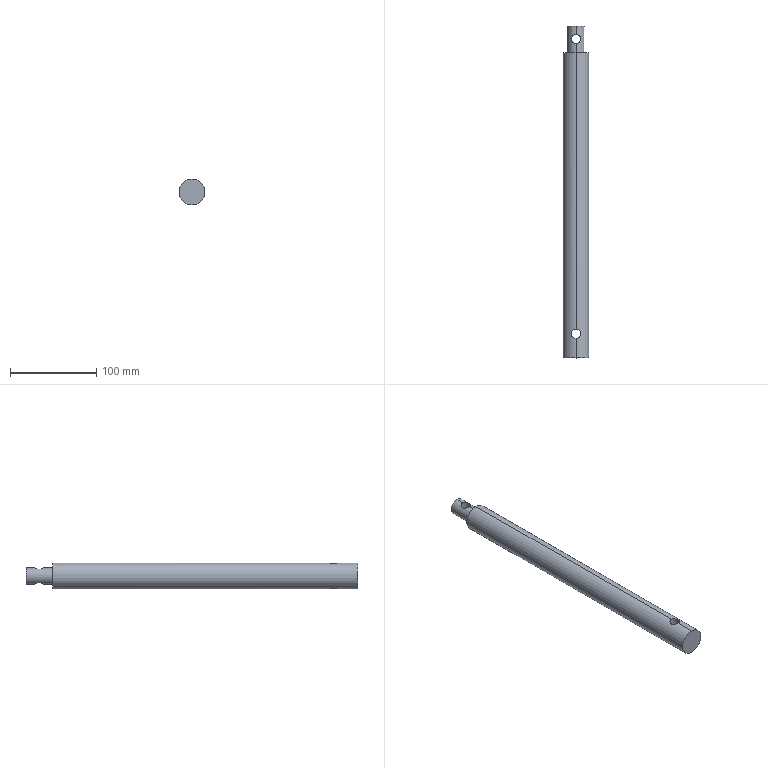Part | SolidWorks | features ICE 2, MoveFace 2, Extrusion 1 | 1 solid | 11 faces | box 30 x 384 x 30 mm | volume 253782 mm3 | cylinder 8 | plane 3 | commonest cylinder face diameters 11 x4 19 x2 30 x2
STEP:
#1=CARTESIAN_POINT('',(-5.5,330.,-13.955));
#2=VERTEX_POINT('',#1);
#3=CARTESIAN_POINT('',(0.,324.5,-15.));
#4=VERTEX_POINT('',#3);
#5=CARTESIAN_POINT('',(-5.5,330.,-13.955));
#6=CARTESIAN_POINT('',(-5.5,329.818,-13.955));
#7=CARTESIAN_POINT('',(-5.491,329.634,-13.959));
#8=CARTESIAN_POINT('',(-5.455,329.272,-13.973));
#9=CARTESIAN_POINT('',(-5.428,329.093,-13.984));
#10=CARTESIAN_POINT('',(-5.321,328.562,-14.025));
#11=CARTESIAN_POINT('',(-5.215,328.214,-14.065));
#12=CARTESIAN_POINT('',(-4.936,327.547,-14.165));
#13=CARTESIAN_POINT('',(-4.766,327.232,-14.224));
#14=CARTESIAN_POINT('',(-4.368,326.639,-14.352));
#15=CARTESIAN_POINT('',(-4.137,326.358,-14.421));
#16=CARTESIAN_POINT('',(-3.633,325.855,-14.556));
#17=CARTESIAN_POINT('',(-3.358,325.63,-14.622));
#18=CARTESIAN_POINT('',(-2.91,325.33,-14.716));
#19=CARTESIAN_POINT('',(-2.755,325.236,-14.746));
#20=CARTESIAN_POINT('',(-2.438,325.067,-14.801));
#21=CARTESIAN_POINT('',(-2.277,324.99,-14.827));
#22=CARTESIAN_POINT('',(-1.782,324.785,-14.897));
#23=CARTESIAN_POINT('',(-1.44,324.679,-14.935));
#24=CARTESIAN_POINT('',(-0.904,324.572,-14.974));
#25=CARTESIAN_POINT('',(-0.7225,324.545,-14.984));
#26=CARTESIAN_POINT('',(-0.3614,324.509,-14.997));
#27=CARTESIAN_POINT('',(-0.1808,324.5,-15.));
#28=CARTESIAN_POINT('',(0.,324.5,-15.));
#29=B_SPLINE_CURVE_WITH_KNOTS('',3,(#5,#6,#7,#8,#9,#10,#11,#12,#13,#14,#15,#16,#17,#18,#19,#20,#21,#22,#23,#24,#25,#26,#27,#28),.UNSPECIFIED.,.F.,.F.,(4,2,2,2,2,2,2,2,2,2,2,4),(0.02696,0.02751,0.02805,0.02913,0.03022,0.0313,0.03239,0.03293,0.03347,0.03456,0.0351,0.03564),.UNSPECIFIED.);
#30=EDGE_CURVE('',#2,#4,#29,.T.);
#31=ORIENTED_EDGE('',*,*,#30,.F.);
#32=CARTESIAN_POINT('',(-5.5,330.,13.955));
#33=VERTEX_POINT('',#32);
#34=CARTESIAN_POINT('',(-5.5,330.,-240.));
#35=DIRECTION('',(0.,0.,1.));
#36=VECTOR('',#35,1000.);
#37=LINE('',#34,#36);
#38=EDGE_CURVE('',#2,#33,#37,.T.);
#39=ORIENTED_EDGE('',*,*,#38,.T.);
#40=CARTESIAN_POINT('',(0.,324.5,15.));
#41=VERTEX_POINT('',#40);
#42=CARTESIAN_POINT('',(0.,324.5,15.));
#43=CARTESIAN_POINT('',(-0.182,324.5,15.));
#44=CARTESIAN_POINT('',(-0.3661,324.509,14.997));
#45=CARTESIAN_POINT('',(-0.7283,324.545,14.983));
#46=CARTESIAN_POINT('',(-0.9072,324.572,14.974));
#47=CARTESIAN_POINT('',(-1.438,324.679,14.935));
#48=CARTESIAN_POINT('',(-1.786,324.785,14.897));
#49=CARTESIAN_POINT('',(-2.454,325.065,14.802));
#50=CARTESIAN_POINT('',(-2.769,325.235,14.745));
#51=CARTESIAN_POINT('',(-3.363,325.633,14.621));
#52=CARTESIAN_POINT('',(-3.643,325.864,14.553));
#53=CARTESIAN_POINT('',(-4.146,326.369,14.418));
#54=CARTESIAN_POINT('',(-4.372,326.643,14.35));
#55=CARTESIAN_POINT('',(-4.671,327.091,14.254));
#56=CARTESIAN_POINT('',(-4.765,327.247,14.223));
#57=CARTESIAN_POINT('',(-4.934,327.563,14.166));
#58=CARTESIAN_POINT('',(-5.01,327.724,14.139));
#59=CARTESIAN_POINT('',(-5.216,328.218,14.065));
#60=CARTESIAN_POINT('',(-5.321,328.561,14.025));
#61=CARTESIAN_POINT('',(-5.428,329.096,13.983));
#62=CARTESIAN_POINT('',(-5.455,329.277,13.973));
#63=CARTESIAN_POINT('',(-5.491,329.639,13.959));
#64=CARTESIAN_POINT('',(-5.5,329.819,13.955));
#65=CARTESIAN_POINT('',(-5.5,330.,13.955));
#66=B_SPLINE_CURVE_WITH_KNOTS('',3,(#42,#43,#44,#45,#46,#47,#48,#49,#50,#51,#52,#53,#54,#55,#56,#57,#58,#59,#60,#61,#62,#63,#64,#65),.UNSPECIFIED.,.F.,.F.,(4,2,2,2,2,2,2,2,2,2,2,4),(0.02696,0.0275,0.02804,0.02912,0.03021,0.03129,0.03238,0.03292,0.03346,0.03455,0.03509,0.03563),.UNSPECIFIED.);
#67=EDGE_CURVE('',#41,#33,#66,.T.);
#68=ORIENTED_EDGE('',*,*,#67,.F.);
#69=CARTESIAN_POINT('',(5.5,330.,13.955));
#70=VERTEX_POINT('',#69);
#71=CARTESIAN_POINT('',(5.5,330.,13.955));
#72=CARTESIAN_POINT('',(5.5,329.634,13.955));
#73=CARTESIAN_POINT('',(5.464,329.275,13.97));
#74=CARTESIAN_POINT('',(5.322,328.566,14.024));
#75=CARTESIAN_POINT('',(5.214,328.214,14.065));
#76=CARTESIAN_POINT('',(4.938,327.551,14.165));
#77=CARTESIAN_POINT('',(4.769,327.236,14.223));
#78=CARTESIAN_POINT('',(4.368,326.638,14.352));
#79=CARTESIAN_POINT('',(4.14,326.361,14.42));
#80=CARTESIAN_POINT('',(3.763,325.984,14.521));
#81=CARTESIAN_POINT('',(3.631,325.865,14.555));
#82=CARTESIAN_POINT('',(3.354,325.638,14.621));
#83=CARTESIAN_POINT('',(3.209,325.529,14.654));
#84=CARTESIAN_POINT('',(2.761,325.23,14.747));
#85=CARTESIAN_POINT('',(2.447,325.061,14.803));
#86=CARTESIAN_POINT('',(1.784,324.785,14.897));
#87=CARTESIAN_POINT('',(1.432,324.677,14.936));
#88=CARTESIAN_POINT('',(0.7232,324.536,14.987));
#89=CARTESIAN_POINT('',(0.364,324.5,15.));
#90=CARTESIAN_POINT('',(0.,324.5,15.));
#91=B_SPLINE_CURVE_WITH_KNOTS('',3,(#71,#72,#73,#74,#75,#76,#77,#78,#79,#80,#81,#82,#83,#84,#85,#86,#87,#88,#89,#90),.UNSPECIFIED.,.F.,.F.,(4,2,2,2,2,2,2,2,2,4),(0.01828,0.01936,0.02045,0.02153,0.02262,0.02316,0.0237,0.02479,0.02587,0.02696),.UNSPECIFIED.);
#92=EDGE_CURVE('',#70,#41,#91,.T.);
#93=ORIENTED_EDGE('',*,*,#92,.F.);
#94=CARTESIAN_POINT('',(5.5,330.,-13.955));
#95=VERTEX_POINT('',#94);
#96=CARTESIAN_POINT('',(5.5,330.,-240.));
#97=DIRECTION('',(0.,0.,1.));
#98=VECTOR('',#97,1000.);
#99=LINE('',#96,#98);
#100=EDGE_CURVE('',#95,#70,#99,.T.);
#101=ORIENTED_EDGE('',*,*,#100,.F.);
#102=CARTESIAN_POINT('',(0.,324.5,-15.));
#103=CARTESIAN_POINT('',(0.1807,324.5,-15.));
#104=CARTESIAN_POINT('',(0.3616,324.509,-14.997));
#105=CARTESIAN_POINT('',(0.7235,324.545,-14.984));
#106=CARTESIAN_POINT('',(0.9054,324.572,-14.974));
#107=CARTESIAN_POINT('',(1.439,324.679,-14.935));
#108=CARTESIAN_POINT('',(1.783,324.785,-14.897));
#109=CARTESIAN_POINT('',(2.448,325.062,-14.803));
#110=CARTESIAN_POINT('',(2.769,325.235,-14.745));
#111=CARTESIAN_POINT('',(3.361,325.632,-14.622));
#112=CARTESIAN_POINT('',(3.637,325.858,-14.555));
#113=CARTESIAN_POINT('',(4.145,326.368,-14.418));
#114=CARTESIAN_POINT('',(4.371,326.643,-14.35));
#115=CARTESIAN_POINT('',(4.668,327.086,-14.255));
#116=CARTESIAN_POINT('',(4.76,327.239,-14.225));
#117=CARTESIAN_POINT('',(4.93,327.556,-14.167));
#118=CARTESIAN_POINT('',(5.009,327.72,-14.139));
#119=CARTESIAN_POINT('',(5.216,328.219,-14.065));
#120=CARTESIAN_POINT('',(5.321,328.562,-14.025));
#121=CARTESIAN_POINT('',(5.463,329.27,-13.97));
#122=CARTESIAN_POINT('',(5.5,329.638,-13.955));
#123=CARTESIAN_POINT('',(5.5,330.,-13.955));
#124=B_SPLINE_CURVE_WITH_KNOTS('',3,(#102,#103,#104,#105,#106,#107,#108,#109,#110,#111,#112,#113,#114,#115,#116,#117,#118,#119,#120,#121,#122,#123),.UNSPECIFIED.,.F.,.F.,(4,2,2,2,2,2,2,2,2,2,4),(0.0009354,0.001478,0.00202,0.003104,0.004189,0.005273,0.006357,0.006899,0.007442,0.008526,0.00961),.UNSPECIFIED.);
#125=EDGE_CURVE('',#4,#95,#124,.T.);
#126=ORIENTED_EDGE('',*,*,#125,.F.);
#127=EDGE_LOOP('',(#31,#39,#68,#93,#101,#126));
#128=FACE_OUTER_BOUND('',#127,.T.);
#129=CARTESIAN_POINT('',(0.,330.,-240.));
#130=DIRECTION('',(0.,0.,1.));
#131=DIRECTION('',(1.,0.,0.));
#132=AXIS2_PLACEMENT_3D('',#129,#130,#131);
#133=CYLINDRICAL_SURFACE('',#132,5.5);
#134=ADVANCED_FACE('',(#128),#133,.F.);
#135=CARTESIAN_POINT('',(-5.5,671.,-7.746));
#136=VERTEX_POINT('',#135);
#137=CARTESIAN_POINT('',(0.,665.5,-9.5));
#138=VERTEX_POINT('',#137);
#139=CARTESIAN_POINT('',(-5.5,671.,-7.746));
#140=CARTESIAN_POINT('',(-5.5,670.628,-7.746));
#141=CARTESIAN_POINT('',(-5.463,670.263,-7.773));
#142=CARTESIAN_POINT('',(-5.317,669.547,-7.873));
#143=CARTESIAN_POINT('',(-5.208,669.195,-7.947));
#144=CARTESIAN_POINT('',(-4.93,668.535,-8.122));
#145=CARTESIAN_POINT('',(-4.759,668.22,-8.225));
#146=CARTESIAN_POINT('',(-4.363,667.633,-8.442));
#147=CARTESIAN_POINT('',(-4.141,667.363,-8.555));
#148=CARTESIAN_POINT('',(-3.644,666.865,-8.778));
#149=CARTESIAN_POINT('',(-3.368,666.637,-8.888));
#150=CARTESIAN_POINT('',(-2.782,666.242,-9.089));
#151=CARTESIAN_POINT('',(-2.47,666.073,-9.18));
#152=CARTESIAN_POINT('',(-1.971,665.862,-9.295));
#153=CARTESIAN_POINT('',(-1.798,665.799,-9.33));
#154=CARTESIAN_POINT('',(-1.449,665.691,-9.39));
#155=CARTESIAN_POINT('',(-1.273,665.646,-9.416));
#156=CARTESIAN_POINT('',(-0.7385,665.538,-9.478));
#157=CARTESIAN_POINT('',(-0.3726,665.5,-9.5));
#158=CARTESIAN_POINT('',(0.,665.5,-9.5));
#159=B_SPLINE_CURVE_WITH_KNOTS('',3,(#139,#140,#141,#142,#143,#144,#145,#146,#147,#148,#149,#150,#151,#152,#153,#154,#155,#156,#157,#158),.UNSPECIFIED.,.F.,.F.,(4,2,2,2,2,2,2,2,2,4),(0.008806,0.009907,0.01101,0.01211,0.01321,0.01431,0.01541,0.01596,0.01651,0.01761),.UNSPECIFIED.);
#160=EDGE_CURVE('',#136,#138,#159,.T.);
#161=ORIENTED_EDGE('',*,*,#160,.F.);
#162=CARTESIAN_POINT('',(-5.5,671.,7.746));
#163=VERTEX_POINT('',#162);
#164=CARTESIAN_POINT('',(-5.5,671.,-240.));
#165=DIRECTION('',(0.,0.,1.));
#166=VECTOR('',#165,1000.);
#167=LINE('',#164,#166);
#168=EDGE_CURVE('',#136,#163,#167,.T.);
#169=ORIENTED_EDGE('',*,*,#168,.T.);
#170=CARTESIAN_POINT('',(0.,665.5,9.5));
#171=VERTEX_POINT('',#170);
#172=CARTESIAN_POINT('',(0.,665.5,9.5));
#173=CARTESIAN_POINT('',(-0.1848,665.5,9.5));
#174=CARTESIAN_POINT('',(-0.3717,665.509,9.495));
#175=CARTESIAN_POINT('',(-0.7383,665.547,9.473));
#176=CARTESIAN_POINT('',(-0.9194,665.574,9.457));
#177=CARTESIAN_POINT('',(-1.277,665.647,9.416));
#178=CARTESIAN_POINT('',(-1.454,665.692,9.39));
#179=CARTESIAN_POINT('',(-1.802,665.801,9.329));
#180=CARTESIAN_POINT('',(-1.975,665.864,9.294));
#181=CARTESIAN_POINT('',(-2.474,666.074,9.179));
#182=CARTESIAN_POINT('',(-2.787,666.245,9.087));
#183=CARTESIAN_POINT('',(-3.377,666.644,8.885));
#184=CARTESIAN_POINT('',(-3.65,666.871,8.775));
#185=CARTESIAN_POINT('',(-4.145,667.368,8.552));
#186=CARTESIAN_POINT('',(-4.37,667.641,8.438));
#187=CARTESIAN_POINT('',(-4.764,668.229,8.222));
#188=CARTESIAN_POINT('',(-4.932,668.539,8.121));
#189=CARTESIAN_POINT('',(-5.139,669.031,7.991));
#190=CARTESIAN_POINT('',(-5.2,669.2,7.951));
#191=CARTESIAN_POINT('',(-5.308,669.547,7.879));
#192=CARTESIAN_POINT('',(-5.353,669.725,7.848));
#193=CARTESIAN_POINT('',(-5.463,670.263,7.773));
#194=CARTESIAN_POINT('',(-5.5,670.628,7.746));
#195=CARTESIAN_POINT('',(-5.5,671.,7.746));
#196=B_SPLINE_CURVE_WITH_KNOTS('',3,(#172,#173,#174,#175,#176,#177,#178,#179,#180,#181,#182,#183,#184,#185,#186,#187,#188,#189,#190,#191,#192,#193,#194,#195),.UNSPECIFIED.,.F.,.F.,(4,2,2,2,2,2,2,2,2,2,2,4),(0.00881,0.00936,0.009909,0.01046,0.01101,0.01211,0.01321,0.01431,0.01541,0.01595,0.0165,0.0176),.UNSPECIFIED.);
#197=EDGE_CURVE('',#171,#163,#196,.T.);
#198=ORIENTED_EDGE('',*,*,#197,.F.);
#199=CARTESIAN_POINT('',(5.5,671.,7.746));
#200=VERTEX_POINT('',#199);
#201=CARTESIAN_POINT('',(5.5,671.,7.746));
#202=CARTESIAN_POINT('',(5.5,670.627,7.746));
#203=CARTESIAN_POINT('',(5.462,670.262,7.773));
#204=CARTESIAN_POINT('',(5.317,669.548,7.873));
#205=CARTESIAN_POINT('',(5.208,669.196,7.947));
#206=CARTESIAN_POINT('',(4.93,668.535,8.122));
#207=CARTESIAN_POINT('',(4.761,668.224,8.224));
#208=CARTESIAN_POINT('',(4.363,667.633,8.442));
#209=CARTESIAN_POINT('',(4.14,667.362,8.555));
#210=CARTESIAN_POINT('',(3.768,666.99,8.722));
#211=CARTESIAN_POINT('',(3.638,666.871,8.777));
#212=CARTESIAN_POINT('',(3.365,666.646,8.885));
#213=CARTESIAN_POINT('',(3.221,666.538,8.939));
#214=CARTESIAN_POINT('',(2.78,666.241,9.09));
#215=CARTESIAN_POINT('',(2.468,666.072,9.18));
#216=CARTESIAN_POINT('',(1.805,665.792,9.333));
#217=CARTESIAN_POINT('',(1.451,665.682,9.396));
#218=CARTESIAN_POINT('',(0.7344,665.537,9.478));
#219=CARTESIAN_POINT('',(0.3703,665.5,9.5));
#220=CARTESIAN_POINT('',(0.,665.5,9.5));
#221=B_SPLINE_CURVE_WITH_KNOTS('',3,(#201,#202,#203,#204,#205,#206,#207,#208,#209,#210,#211,#212,#213,#214,#215,#216,#217,#218,#219,#220),.UNSPECIFIED.,.F.,.F.,(4,2,2,2,2,2,2,2,2,4),(0.,0.001101,0.002203,0.003304,0.004405,0.004956,0.005506,0.006608,0.007709,0.00881),.UNSPECIFIED.);
#222=EDGE_CURVE('',#200,#171,#221,.T.);
#223=ORIENTED_EDGE('',*,*,#222,.F.);
#224=CARTESIAN_POINT('',(5.5,671.,-7.746));
#225=VERTEX_POINT('',#224);
#226=CARTESIAN_POINT('',(5.5,671.,-240.));
#227=DIRECTION('',(0.,0.,1.));
#228=VECTOR('',#227,1000.);
#229=LINE('',#226,#228);
#230=EDGE_CURVE('',#225,#200,#229,.T.);
#231=ORIENTED_EDGE('',*,*,#230,.F.);
#232=CARTESIAN_POINT('',(0.,665.5,-9.5));
#233=CARTESIAN_POINT('',(0.372,665.5,-9.5));
#234=CARTESIAN_POINT('',(0.7369,665.537,-9.478));
#235=CARTESIAN_POINT('',(1.453,665.683,-9.395));
#236=CARTESIAN_POINT('',(1.807,665.793,-9.333));
#237=CARTESIAN_POINT('',(2.471,666.073,-9.179));
#238=CARTESIAN_POINT('',(2.785,666.244,-9.088));
#239=CARTESIAN_POINT('',(3.377,666.644,-8.885));
#240=CARTESIAN_POINT('',(3.648,666.869,-8.776));
#241=CARTESIAN_POINT('',(4.143,667.366,-8.553));
#242=CARTESIAN_POINT('',(4.369,667.641,-8.439));
#243=CARTESIAN_POINT('',(4.762,668.225,-8.224));
#244=CARTESIAN_POINT('',(4.929,668.535,-8.123));
#245=CARTESIAN_POINT('',(5.207,669.194,-7.947));
#246=CARTESIAN_POINT('',(5.317,669.545,-7.873));
#247=CARTESIAN_POINT('',(5.426,670.081,-7.798));
#248=CARTESIAN_POINT('',(5.453,670.262,-7.779));
#249=CARTESIAN_POINT('',(5.49,670.628,-7.753));
#250=CARTESIAN_POINT('',(5.5,670.815,-7.746));
#251=CARTESIAN_POINT('',(5.5,671.,-7.746));
#252=B_SPLINE_CURVE_WITH_KNOTS('',3,(#232,#233,#234,#235,#236,#237,#238,#239,#240,#241,#242,#243,#244,#245,#246,#247,#248,#249,#250,#251),.UNSPECIFIED.,.F.,.F.,(4,2,2,2,2,2,2,2,2,4),(0.01761,0.01871,0.01981,0.02091,0.022,0.0231,0.0242,0.0253,0.02585,0.0264),.UNSPECIFIED.);
#253=EDGE_CURVE('',#138,#225,#252,.T.);
#254=ORIENTED_EDGE('',*,*,#253,.F.);
#255=EDGE_LOOP('',(#161,#169,#198,#223,#231,#254));
#256=FACE_OUTER_BOUND('',#255,.T.);
#257=CARTESIAN_POINT('',(0.,671.,-240.));
#258=DIRECTION('',(0.,0.,1.));
#259=DIRECTION('',(1.,0.,0.));
#260=AXIS2_PLACEMENT_3D('',#257,#258,#259);
#261=CYLINDRICAL_SURFACE('',#260,5.5);
#262=ADVANCED_FACE('',(#256),#261,.F.);
#263=CARTESIAN_POINT('',(0.,686.,9.5));
#264=VERTEX_POINT('',#263);
#265=CARTESIAN_POINT('',(0.,686.,-9.5));
#266=VERTEX_POINT('',#265);
#267=CARTESIAN_POINT('',(0.,686.,0.));
#268=DIRECTION('',(0.,1.,0.));
#269=DIRECTION('',(0.,0.,1.));
#270=AXIS2_PLACEMENT_3D('',#267,#268,#269);
#271=CIRCLE('',#270,9.5);
#272=EDGE_CURVE('',#264,#266,#271,.T.);
#273=ORIENTED_EDGE('',*,*,#272,.F.);
#274=CARTESIAN_POINT('',(0.,676.5,9.5));
#275=VERTEX_POINT('',#274);
#276=CARTESIAN_POINT('',(0.,686.,9.5));
#277=DIRECTION('',(0.,-1.,0.));
#278=VECTOR('',#277,1000.);
#279=LINE('',#276,#278);
#280=EDGE_CURVE('',#264,#275,#279,.T.);
#281=ORIENTED_EDGE('',*,*,#280,.T.);
#282=CARTESIAN_POINT('',(0.,676.5,9.5));
#283=CARTESIAN_POINT('',(0.3713,676.5,9.5));
#284=CARTESIAN_POINT('',(0.7393,676.462,9.478));
#285=CARTESIAN_POINT('',(1.455,676.317,9.395));
#286=CARTESIAN_POINT('',(1.808,676.207,9.333));
#287=CARTESIAN_POINT('',(2.473,675.926,9.179));
#288=CARTESIAN_POINT('',(2.786,675.756,9.088));
#289=CARTESIAN_POINT('',(3.378,675.355,8.885));
#290=CARTESIAN_POINT('',(3.65,675.129,8.775));
#291=CARTESIAN_POINT('',(4.021,674.757,8.608));
#292=CARTESIAN_POINT('',(4.139,674.627,8.552));
#293=CARTESIAN_POINT('',(4.362,674.354,8.44));
#294=CARTESIAN_POINT('',(4.469,674.211,8.384));
#295=CARTESIAN_POINT('',(4.763,673.772,8.223));
#296=CARTESIAN_POINT('',(4.931,673.462,8.122));
#297=CARTESIAN_POINT('',(5.208,672.805,7.947));
#298=CARTESIAN_POINT('',(5.317,672.453,7.873));
#299=CARTESIAN_POINT('',(5.462,671.738,7.773));
#300=CARTESIAN_POINT('',(5.5,671.372,7.746));
#301=CARTESIAN_POINT('',(5.5,671.,7.746));
#302=B_SPLINE_CURVE_WITH_KNOTS('',3,(#282,#283,#284,#285,#286,#287,#288,#289,#290,#291,#292,#293,#294,#295,#296,#297,#298,#299,#300,#301),.UNSPECIFIED.,.F.,.F.,(4,2,2,2,2,2,2,2,2,4),(0.02639,0.02749,0.02859,0.02969,0.03078,0.03133,0.03188,0.03298,0.03408,0.03517),.UNSPECIFIED.);
#303=EDGE_CURVE('',#275,#200,#302,.T.);
#304=ORIENTED_EDGE('',*,*,#303,.T.);
#305=ORIENTED_EDGE('',*,*,#222,.T.);
#306=CARTESIAN_POINT('',(0.,655.,9.5));
#307=VERTEX_POINT('',#306);
#308=CARTESIAN_POINT('',(0.,686.,9.5));
#309=DIRECTION('',(0.,-1.,0.));
#310=VECTOR('',#309,1000.);
#311=LINE('',#308,#310);
#312=EDGE_CURVE('',#171,#307,#311,.T.);
#313=ORIENTED_EDGE('',*,*,#312,.T.);
#314=CARTESIAN_POINT('',(0.,655.,-9.5));
#315=VERTEX_POINT('',#314);
#316=CARTESIAN_POINT('',(0.,655.,0.));
#317=DIRECTION('',(0.,1.,0.));
#318=DIRECTION('',(0.,0.,1.));
#319=AXIS2_PLACEMENT_3D('',#316,#317,#318);
#320=CIRCLE('',#319,9.5);
#321=EDGE_CURVE('',#307,#315,#320,.T.);
#322=ORIENTED_EDGE('',*,*,#321,.T.);
#323=CARTESIAN_POINT('',(0.,686.,-9.5));
#324=DIRECTION('',(0.,-1.,0.));
#325=VECTOR('',#324,1000.);
#326=LINE('',#323,#325);
#327=EDGE_CURVE('',#138,#315,#326,.T.);
#328=ORIENTED_EDGE('',*,*,#327,.F.);
#329=ORIENTED_EDGE('',*,*,#253,.T.);
#330=CARTESIAN_POINT('',(0.,676.5,-9.5));
#331=VERTEX_POINT('',#330);
#332=CARTESIAN_POINT('',(5.5,671.,-7.746));
#333=CARTESIAN_POINT('',(5.5,671.37,-7.746));
#334=CARTESIAN_POINT('',(5.463,671.734,-7.773));
#335=CARTESIAN_POINT('',(5.354,672.272,-7.848));
#336=CARTESIAN_POINT('',(5.308,672.451,-7.879));
#337=CARTESIAN_POINT('',(5.201,672.797,-7.95));
#338=CARTESIAN_POINT('',(5.14,672.966,-7.99));
#339=CARTESIAN_POINT('',(4.932,673.461,-8.121));
#340=CARTESIAN_POINT('',(4.76,673.777,-8.224));
#341=CARTESIAN_POINT('',(4.367,674.363,-8.44));
#342=CARTESIAN_POINT('',(4.144,674.633,-8.553));
#343=CARTESIAN_POINT('',(3.771,675.007,-8.72));
#344=CARTESIAN_POINT('',(3.64,675.127,-8.776));
#345=CARTESIAN_POINT('',(3.368,675.352,-8.884));
#346=CARTESIAN_POINT('',(3.227,675.457,-8.937));
#347=CARTESIAN_POINT('',(2.789,675.754,-9.087));
#348=CARTESIAN_POINT('',(2.477,675.924,-9.178));
#349=CARTESIAN_POINT('',(1.809,676.207,-9.333));
#350=CARTESIAN_POINT('',(1.46,676.315,-9.394));
#351=CARTESIAN_POINT('',(0.7444,676.462,-9.478));
#352=CARTESIAN_POINT('',(0.3717,676.5,-9.5));
#353=CARTESIAN_POINT('',(0.,676.5,-9.5));
#354=B_SPLINE_CURVE_WITH_KNOTS('',3,(#332,#333,#334,#335,#336,#337,#338,#339,#340,#341,#342,#343,#344,#345,#346,#347,#348,#349,#350,#351,#352,#353),.UNSPECIFIED.,.F.,.F.,(4,2,2,2,2,2,2,2,2,2,4),(0.0264,0.0275,0.02804,0.02859,0.02969,0.03079,0.03134,0.03189,0.03298,0.03408,0.03518),.UNSPECIFIED.);
#355=EDGE_CURVE('',#225,#331,#354,.T.);
#356=ORIENTED_EDGE('',*,*,#355,.T.);
#357=CARTESIAN_POINT('',(0.,686.,-9.5));
#358=DIRECTION('',(0.,-1.,0.));
#359=VECTOR('',#358,1000.);
#360=LINE('',#357,#359);
#361=EDGE_CURVE('',#266,#331,#360,.T.);
#362=ORIENTED_EDGE('',*,*,#361,.F.);
#363=EDGE_LOOP('',(#273,#281,#304,#305,#313,#322,#328,#329,#356,#362));
#364=FACE_OUTER_BOUND('',#363,.T.);
#365=CARTESIAN_POINT('',(0.,686.,0.));
#366=DIRECTION('',(0.,-1.,0.));
#367=DIRECTION('',(0.,0.,-1.));
#368=AXIS2_PLACEMENT_3D('',#365,#366,#367);
#369=CYLINDRICAL_SURFACE('',#368,9.5);
#370=ADVANCED_FACE('',(#364),#369,.T.);
#371=CARTESIAN_POINT('',(0.,655.,15.));
#372=VERTEX_POINT('',#371);
#373=CARTESIAN_POINT('',(0.,655.,-15.));
#374=VERTEX_POINT('',#373);
#375=CARTESIAN_POINT('',(0.,655.,0.));
#376=DIRECTION('',(0.,1.,0.));
#377=DIRECTION('',(0.,0.,1.));
#378=AXIS2_PLACEMENT_3D('',#375,#376,#377);
#379=CIRCLE('',#378,15.);
#380=EDGE_CURVE('',#372,#374,#379,.T.);
#381=ORIENTED_EDGE('',*,*,#380,.F.);
#382=CARTESIAN_POINT('',(0.,335.5,15.));
#383=VERTEX_POINT('',#382);
#384=CARTESIAN_POINT('',(0.,656.,15.));
#385=DIRECTION('',(0.,-1.,0.));
#386=VECTOR('',#385,1000.);
#387=LINE('',#384,#386);
#388=EDGE_CURVE('',#372,#383,#387,.T.);
#389=ORIENTED_EDGE('',*,*,#388,.T.);
#390=CARTESIAN_POINT('',(0.,335.5,15.));
#391=CARTESIAN_POINT('',(0.3621,335.5,15.));
#392=CARTESIAN_POINT('',(0.7219,335.465,14.987));
#393=CARTESIAN_POINT('',(1.258,335.357,14.948));
#394=CARTESIAN_POINT('',(1.435,335.313,14.932));
#395=CARTESIAN_POINT('',(1.781,335.207,14.895));
#396=CARTESIAN_POINT('',(1.95,335.146,14.874));
#397=CARTESIAN_POINT('',(2.281,335.008,14.826));
#398=CARTESIAN_POINT('',(2.443,334.931,14.801));
#399=CARTESIAN_POINT('',(2.76,334.76,14.745));
#400=CARTESIAN_POINT('',(2.916,334.667,14.715));
#401=CARTESIAN_POINT('',(3.363,334.367,14.621));
#402=CARTESIAN_POINT('',(3.637,334.141,14.555));
#403=CARTESIAN_POINT('',(4.142,333.636,14.419));
#404=CARTESIAN_POINT('',(4.372,333.356,14.35));
#405=CARTESIAN_POINT('',(4.768,332.764,14.223));
#406=CARTESIAN_POINT('',(4.937,332.45,14.165));
#407=CARTESIAN_POINT('',(5.146,331.949,14.09));
#408=CARTESIAN_POINT('',(5.208,331.778,14.067));
#409=CARTESIAN_POINT('',(5.313,331.433,14.028));
#410=CARTESIAN_POINT('',(5.401,331.084,13.994));
#411=CARTESIAN_POINT('',(5.455,330.727,13.973));
#412=CARTESIAN_POINT('',(5.491,330.366,13.959));
#413=CARTESIAN_POINT('',(5.5,330.183,13.955));
#414=CARTESIAN_POINT('',(5.5,330.,13.955));
#415=B_SPLINE_CURVE_WITH_KNOTS('',3,(#390,#391,#392,#393,#394,#395,#396,#397,#398,#399,#400,#401,#402,#403,#404,#405,#406,#407,#408,#409,#410,#411,#412,#413,#414),.UNSPECIFIED.,.F.,.F.,(4,2,2,2,2,2,2,2,2,2,1,2,4),(0.009602,0.01069,0.01123,0.01177,0.01231,0.01286,0.01394,0.01503,0.01611,0.01665,0.01719,0.01774,0.01828),.UNSPECIFIED.);
#416=EDGE_CURVE('',#383,#70,#415,.T.);
#417=ORIENTED_EDGE('',*,*,#416,.T.);
#418=ORIENTED_EDGE('',*,*,#92,.T.);
#419=CARTESIAN_POINT('',(0.,302.,15.));
#420=VERTEX_POINT('',#419);
#421=CARTESIAN_POINT('',(0.,656.,15.));
#422=DIRECTION('',(0.,-1.,0.));
#423=VECTOR('',#422,1000.);
#424=LINE('',#421,#423);
#425=EDGE_CURVE('',#41,#420,#424,.T.);
#426=ORIENTED_EDGE('',*,*,#425,.T.);
#427=CARTESIAN_POINT('',(0.,302.,-15.));
#428=VERTEX_POINT('',#427);
#429=CARTESIAN_POINT('',(0.,302.,0.));
#430=DIRECTION('',(0.,1.,0.));
#431=DIRECTION('',(0.,0.,1.));
#432=AXIS2_PLACEMENT_3D('',#429,#430,#431);
#433=CIRCLE('',#432,15.);
#434=EDGE_CURVE('',#420,#428,#433,.T.);
#435=ORIENTED_EDGE('',*,*,#434,.T.);
#436=CARTESIAN_POINT('',(0.,656.,-15.));
#437=DIRECTION('',(0.,-1.,0.));
#438=VECTOR('',#437,1000.);
#439=LINE('',#436,#438);
#440=EDGE_CURVE('',#4,#428,#439,.T.);
#441=ORIENTED_EDGE('',*,*,#440,.F.);
#442=ORIENTED_EDGE('',*,*,#125,.T.);
#443=CARTESIAN_POINT('',(0.,335.5,-15.));
#444=VERTEX_POINT('',#443);
#445=CARTESIAN_POINT('',(5.5,330.,-13.955));
#446=CARTESIAN_POINT('',(5.5,330.362,-13.955));
#447=CARTESIAN_POINT('',(5.465,330.722,-13.969));
#448=CARTESIAN_POINT('',(5.357,331.257,-14.011));
#449=CARTESIAN_POINT('',(5.313,331.435,-14.028));
#450=CARTESIAN_POINT('',(5.207,331.78,-14.067));
#451=CARTESIAN_POINT('',(5.146,331.949,-14.09));
#452=CARTESIAN_POINT('',(5.008,332.28,-14.139));
#453=CARTESIAN_POINT('',(4.931,332.442,-14.167));
#454=CARTESIAN_POINT('',(4.761,332.759,-14.225));
#455=CARTESIAN_POINT('',(4.668,332.915,-14.256));
#456=CARTESIAN_POINT('',(4.368,333.361,-14.351));
#457=CARTESIAN_POINT('',(4.142,333.636,-14.419));
#458=CARTESIAN_POINT('',(3.638,334.14,-14.554));
#459=CARTESIAN_POINT('',(3.358,334.371,-14.622));
#460=CARTESIAN_POINT('',(2.765,334.768,-14.746));
#461=CARTESIAN_POINT('',(2.451,334.937,-14.802));
#462=CARTESIAN_POINT('',(1.95,335.146,-14.874));
#463=CARTESIAN_POINT('',(1.778,335.208,-14.895));
#464=CARTESIAN_POINT('',(1.433,335.313,-14.932));
#465=CARTESIAN_POINT('',(1.084,335.401,-14.964));
#466=CARTESIAN_POINT('',(0.7269,335.455,-14.983));
#467=CARTESIAN_POINT('',(0.3661,335.491,-14.997));
#468=CARTESIAN_POINT('',(0.1827,335.5,-15.));
#469=CARTESIAN_POINT('',(0.,335.5,-15.));
#470=B_SPLINE_CURVE_WITH_KNOTS('',3,(#445,#446,#447,#448,#449,#450,#451,#452,#453,#454,#455,#456,#457,#458,#459,#460,#461,#462,#463,#464,#465,#466,#467,#468,#469),.UNSPECIFIED.,.F.,.F.,(4,2,2,2,2,2,2,2,2,2,1,2,4),(0.00961,0.01069,0.01124,0.01178,0.01232,0.01286,0.01395,0.01503,0.01612,0.01666,0.0172,0.01774,0.01829),.UNSPECIFIED.);
#471=EDGE_CURVE('',#95,#444,#470,.T.);
#472=ORIENTED_EDGE('',*,*,#471,.T.);
#473=CARTESIAN_POINT('',(0.,656.,-15.));
#474=DIRECTION('',(0.,-1.,0.));
#475=VECTOR('',#474,1000.);
#476=LINE('',#473,#475);
#477=EDGE_CURVE('',#374,#444,#476,.T.);
#478=ORIENTED_EDGE('',*,*,#477,.F.);
#479=EDGE_LOOP('',(#381,#389,#417,#418,#426,#435,#441,#442,#472,#478));
#480=FACE_OUTER_BOUND('',#479,.T.);
#481=CARTESIAN_POINT('',(0.,656.,0.));
#482=DIRECTION('',(0.,-1.,0.));
#483=DIRECTION('',(0.,0.,-1.));
#484=AXIS2_PLACEMENT_3D('',#481,#482,#483);
#485=CYLINDRICAL_SURFACE('',#484,15.);
#486=ADVANCED_FACE('',(#480),#485,.T.);
#487=ORIENTED_EDGE('',*,*,#388,.F.);
#488=CARTESIAN_POINT('',(0.,655.,0.));
#489=DIRECTION('',(0.,1.,0.));
#490=DIRECTION('',(0.,0.,1.));
#491=AXIS2_PLACEMENT_3D('',#488,#489,#490);
#492=CIRCLE('',#491,15.);
#493=EDGE_CURVE('',#374,#372,#492,.T.);
#494=ORIENTED_EDGE('',*,*,#493,.F.);
#495=ORIENTED_EDGE('',*,*,#477,.T.);
#496=CARTESIAN_POINT('',(0.,335.5,-15.));
#497=CARTESIAN_POINT('',(-0.3655,335.5,-15.));
#498=CARTESIAN_POINT('',(-0.7254,335.464,-14.987));
#499=CARTESIAN_POINT('',(-1.434,335.322,-14.935));
#500=CARTESIAN_POINT('',(-1.786,335.214,-14.897));
#501=CARTESIAN_POINT('',(-2.45,334.937,-14.802));
#502=CARTESIAN_POINT('',(-2.765,334.768,-14.746));
#503=CARTESIAN_POINT('',(-3.363,334.367,-14.621));
#504=CARTESIAN_POINT('',(-3.64,334.138,-14.554));
#505=CARTESIAN_POINT('',(-4.017,333.761,-14.453));
#506=CARTESIAN_POINT('',(-4.137,333.629,-14.419));
#507=CARTESIAN_POINT('',(-4.364,333.353,-14.352));
#508=CARTESIAN_POINT('',(-4.472,333.207,-14.318));
#509=CARTESIAN_POINT('',(-4.771,332.76,-14.223));
#510=CARTESIAN_POINT('',(-4.939,332.445,-14.164));
#511=CARTESIAN_POINT('',(-5.215,331.784,-14.065));
#512=CARTESIAN_POINT('',(-5.323,331.432,-14.024));
#513=CARTESIAN_POINT('',(-5.464,330.723,-13.97));
#514=CARTESIAN_POINT('',(-5.5,330.364,-13.955));
#515=CARTESIAN_POINT('',(-5.5,330.,-13.955));
#516=B_SPLINE_CURVE_WITH_KNOTS('',3,(#496,#497,#498,#499,#500,#501,#502,#503,#504,#505,#506,#507,#508,#509,#510,#511,#512,#513,#514,#515),.UNSPECIFIED.,.F.,.F.,(4,2,2,2,2,2,2,2,2,4),(0.01829,0.01937,0.02046,0.02154,0.02263,0.02317,0.02371,0.02479,0.02588,0.02696),.UNSPECIFIED.);
#517=EDGE_CURVE('',#444,#2,#516,.T.);
#518=ORIENTED_EDGE('',*,*,#517,.T.);
#519=ORIENTED_EDGE('',*,*,#30,.T.);
#520=ORIENTED_EDGE('',*,*,#440,.T.);
#521=CARTESIAN_POINT('',(0.,302.,0.));
#522=DIRECTION('',(0.,1.,0.));
#523=DIRECTION('',(0.,0.,1.));
#524=AXIS2_PLACEMENT_3D('',#521,#522,#523);
#525=CIRCLE('',#524,15.);
#526=EDGE_CURVE('',#428,#420,#525,.T.);
#527=ORIENTED_EDGE('',*,*,#526,.T.);
#528=ORIENTED_EDGE('',*,*,#425,.F.);
#529=ORIENTED_EDGE('',*,*,#67,.T.);
#530=CARTESIAN_POINT('',(-5.5,330.,13.955));
#531=CARTESIAN_POINT('',(-5.5,330.181,13.955));
#532=CARTESIAN_POINT('',(-5.491,330.362,13.959));
#533=CARTESIAN_POINT('',(-5.455,330.723,13.973));
#534=CARTESIAN_POINT('',(-5.428,330.905,13.983));
#535=CARTESIAN_POINT('',(-5.321,331.439,14.025));
#536=CARTESIAN_POINT('',(-5.215,331.783,14.065));
#537=CARTESIAN_POINT('',(-4.939,332.447,14.164));
#538=CARTESIAN_POINT('',(-4.766,332.768,14.224));
#539=CARTESIAN_POINT('',(-4.369,333.36,14.351));
#540=CARTESIAN_POINT('',(-4.143,333.635,14.419));
#541=CARTESIAN_POINT('',(-3.634,334.144,14.556));
#542=CARTESIAN_POINT('',(-3.359,334.37,14.622));
#543=CARTESIAN_POINT('',(-2.915,334.667,14.715));
#544=CARTESIAN_POINT('',(-2.762,334.76,14.744));
#545=CARTESIAN_POINT('',(-2.445,334.93,14.8));
#546=CARTESIAN_POINT('',(-2.281,335.008,14.827));
#547=CARTESIAN_POINT('',(-1.781,335.216,14.898));
#548=CARTESIAN_POINT('',(-1.438,335.321,14.935));
#549=CARTESIAN_POINT('',(-0.7301,335.463,14.986));
#550=CARTESIAN_POINT('',(-0.3621,335.5,15.));
#551=CARTESIAN_POINT('',(0.,335.5,15.));
#552=B_SPLINE_CURVE_WITH_KNOTS('',3,(#530,#531,#532,#533,#534,#535,#536,#537,#538,#539,#540,#541,#542,#543,#544,#545,#546,#547,#548,#549,#550,#551),.UNSPECIFIED.,.F.,.F.,(4,2,2,2,2,2,2,2,2,2,4),(0.0009274,0.00147,0.002012,0.003096,0.00418,0.005265,0.006349,0.006891,0.007434,0.008518,0.009602),.UNSPECIFIED.);
#553=EDGE_CURVE('',#33,#383,#552,.T.);
#554=ORIENTED_EDGE('',*,*,#553,.T.);
#555=EDGE_LOOP('',(#487,#494,#495,#518,#519,#520,#527,#528,#529,#554));
#556=FACE_OUTER_BOUND('',#555,.T.);
#557=CARTESIAN_POINT('',(0.,656.,0.));
#558=DIRECTION('',(0.,-1.,0.));
#559=DIRECTION('',(0.,0.,-1.));
#560=AXIS2_PLACEMENT_3D('',#557,#558,#559);
#561=CYLINDRICAL_SURFACE('',#560,15.);
#562=ADVANCED_FACE('',(#556),#561,.T.);
#563=CARTESIAN_POINT('',(0.,655.,0.));
#564=DIRECTION('',(0.,1.,0.));
#565=DIRECTION('',(0.,0.,1.));
#566=AXIS2_PLACEMENT_3D('',#563,#564,#565);
#567=CIRCLE('',#566,9.5);
#568=EDGE_CURVE('',#315,#307,#567,.T.);
#569=ORIENTED_EDGE('',*,*,#568,.F.);
#570=ORIENTED_EDGE('',*,*,#321,.F.);
#571=EDGE_LOOP('',(#569,#570));
#572=FACE_BOUND('',#571,.T.);
#573=ORIENTED_EDGE('',*,*,#493,.T.);
#574=ORIENTED_EDGE('',*,*,#380,.T.);
#575=EDGE_LOOP('',(#573,#574));
#576=FACE_OUTER_BOUND('',#575,.T.);
#577=CARTESIAN_POINT('',(0.,655.,0.));
#578=DIRECTION('',(0.,1.,0.));
#579=DIRECTION('',(0.,0.,1.));
#580=AXIS2_PLACEMENT_3D('',#577,#578,#579);
#581=PLANE('',#580);
#582=ADVANCED_FACE('',(#572,#576),#581,.T.);
#583=ORIENTED_EDGE('',*,*,#526,.F.);
#584=ORIENTED_EDGE('',*,*,#434,.F.);
#585=EDGE_LOOP('',(#583,#584));
#586=FACE_OUTER_BOUND('',#585,.T.);
#587=CARTESIAN_POINT('',(0.,302.,0.));
#588=DIRECTION('',(0.,1.,0.));
#589=DIRECTION('',(0.,0.,1.));
#590=AXIS2_PLACEMENT_3D('',#587,#588,#589);
#591=PLANE('',#590);
#592=ADVANCED_FACE('',(#586),#591,.F.);
#593=ORIENTED_EDGE('',*,*,#280,.F.);
#594=CARTESIAN_POINT('',(0.,686.,0.));
#595=DIRECTION('',(0.,1.,0.));
#596=DIRECTION('',(0.,0.,1.));
#597=AXIS2_PLACEMENT_3D('',#594,#595,#596);
#598=CIRCLE('',#597,9.5);
#599=EDGE_CURVE('',#266,#264,#598,.T.);
#600=ORIENTED_EDGE('',*,*,#599,.F.);
#601=ORIENTED_EDGE('',*,*,#361,.T.);
#602=CARTESIAN_POINT('',(0.,676.5,-9.5));
#603=CARTESIAN_POINT('',(-0.3727,676.5,-9.5));
#604=CARTESIAN_POINT('',(-0.7377,676.463,-9.478));
#605=CARTESIAN_POINT('',(-1.453,676.317,-9.395));
#606=CARTESIAN_POINT('',(-1.807,676.207,-9.333));
#607=CARTESIAN_POINT('',(-2.471,675.927,-9.179));
#608=CARTESIAN_POINT('',(-2.784,675.757,-9.088));
#609=CARTESIAN_POINT('',(-3.376,675.356,-8.885));
#610=CARTESIAN_POINT('',(-3.648,675.131,-8.776));
#611=CARTESIAN_POINT('',(-4.019,674.758,-8.609));
#612=CARTESIAN_POINT('',(-4.137,674.628,-8.553));
#613=CARTESIAN_POINT('',(-4.361,674.356,-8.441));
#614=CARTESIAN_POINT('',(-4.467,674.213,-8.385));
#615=CARTESIAN_POINT('',(-4.763,673.774,-8.223));
#616=CARTESIAN_POINT('',(-4.93,673.464,-8.122));
#617=CARTESIAN_POINT('',(-5.207,672.807,-7.948));
#618=CARTESIAN_POINT('',(-5.317,672.454,-7.873));
#619=CARTESIAN_POINT('',(-5.462,671.739,-7.773));
#620=CARTESIAN_POINT('',(-5.5,671.372,-7.746));
#621=CARTESIAN_POINT('',(-5.5,671.,-7.746));
#622=B_SPLINE_CURVE_WITH_KNOTS('',3,(#602,#603,#604,#605,#606,#607,#608,#609,#610,#611,#612,#613,#614,#615,#616,#617,#618,#619,#620,#621),.UNSPECIFIED.,.F.,.F.,(4,2,2,2,2,2,2,2,2,4),(0.,0.001101,0.002202,0.003302,0.004403,0.004954,0.005504,0.006605,0.007705,0.008806),.UNSPECIFIED.);
#623=EDGE_CURVE('',#331,#136,#622,.T.);
#624=ORIENTED_EDGE('',*,*,#623,.T.);
#625=ORIENTED_EDGE('',*,*,#160,.T.);
#626=ORIENTED_EDGE('',*,*,#327,.T.);
#627=ORIENTED_EDGE('',*,*,#568,.T.);
#628=ORIENTED_EDGE('',*,*,#312,.F.);
#629=ORIENTED_EDGE('',*,*,#197,.T.);
#630=CARTESIAN_POINT('',(-5.5,671.,7.746));
#631=CARTESIAN_POINT('',(-5.5,671.372,7.746));
#632=CARTESIAN_POINT('',(-5.462,671.739,7.773));
#633=CARTESIAN_POINT('',(-5.317,672.454,7.873));
#634=CARTESIAN_POINT('',(-5.207,672.806,7.947));
#635=CARTESIAN_POINT('',(-4.929,673.466,8.123));
#636=CARTESIAN_POINT('',(-4.759,673.78,8.225));
#637=CARTESIAN_POINT('',(-4.362,674.368,8.442));
#638=CARTESIAN_POINT('',(-4.139,674.639,8.555));
#639=CARTESIAN_POINT('',(-3.643,675.135,8.778));
#640=CARTESIAN_POINT('',(-3.367,675.363,8.889));
#641=CARTESIAN_POINT('',(-2.78,675.759,9.089));
#642=CARTESIAN_POINT('',(-2.468,675.928,9.18));
#643=CARTESIAN_POINT('',(-1.804,676.208,9.333));
#644=CARTESIAN_POINT('',(-1.45,676.318,9.396));
#645=CARTESIAN_POINT('',(-0.7359,676.463,9.478));
#646=CARTESIAN_POINT('',(-0.3718,676.5,9.5));
#647=CARTESIAN_POINT('',(0.,676.5,9.5));
#648=B_SPLINE_CURVE_WITH_KNOTS('',3,(#630,#631,#632,#633,#634,#635,#636,#637,#638,#639,#640,#641,#642,#643,#644,#645,#646,#647),.UNSPECIFIED.,.F.,.F.,(4,2,2,2,2,2,2,2,4),(0.0176,0.0187,0.0198,0.0209,0.022,0.0231,0.0242,0.0253,0.02639),.UNSPECIFIED.);
#649=EDGE_CURVE('',#163,#275,#648,.T.);
#650=ORIENTED_EDGE('',*,*,#649,.T.);
#651=EDGE_LOOP('',(#593,#600,#601,#624,#625,#626,#627,#628,#629,#650));
#652=FACE_OUTER_BOUND('',#651,.T.);
#653=CARTESIAN_POINT('',(0.,686.,0.));
#654=DIRECTION('',(0.,-1.,0.));
#655=DIRECTION('',(0.,0.,-1.));
#656=AXIS2_PLACEMENT_3D('',#653,#654,#655);
#657=CYLINDRICAL_SURFACE('',#656,9.5);
#658=ADVANCED_FACE('',(#652),#657,.T.);
#659=ORIENTED_EDGE('',*,*,#599,.T.);
#660=ORIENTED_EDGE('',*,*,#272,.T.);
#661=EDGE_LOOP('',(#659,#660));
#662=FACE_OUTER_BOUND('',#661,.T.);
#663=CARTESIAN_POINT('',(0.,686.,0.));
#664=DIRECTION('',(0.,1.,0.));
#665=DIRECTION('',(0.,0.,1.));
#666=AXIS2_PLACEMENT_3D('',#663,#664,#665);
#667=PLANE('',#666);
#668=ADVANCED_FACE('',(#662),#667,.T.);
#669=ORIENTED_EDGE('',*,*,#168,.F.);
#670=ORIENTED_EDGE('',*,*,#623,.F.);
#671=ORIENTED_EDGE('',*,*,#355,.F.);
#672=ORIENTED_EDGE('',*,*,#230,.T.);
#673=ORIENTED_EDGE('',*,*,#303,.F.);
#674=ORIENTED_EDGE('',*,*,#649,.F.);
#675=EDGE_LOOP('',(#669,#670,#671,#672,#673,#674));
#676=FACE_OUTER_BOUND('',#675,.T.);
#677=CARTESIAN_POINT('',(0.,671.,-240.));
#678=DIRECTION('',(0.,0.,1.));
#679=DIRECTION('',(1.,0.,0.));
#680=AXIS2_PLACEMENT_3D('',#677,#678,#679);
#681=CYLINDRICAL_SURFACE('',#680,5.5);
#682=ADVANCED_FACE('',(#676),#681,.F.);
#683=ORIENTED_EDGE('',*,*,#38,.F.);
#684=ORIENTED_EDGE('',*,*,#517,.F.);
#685=ORIENTED_EDGE('',*,*,#471,.F.);
#686=ORIENTED_EDGE('',*,*,#100,.T.);
#687=ORIENTED_EDGE('',*,*,#416,.F.);
#688=ORIENTED_EDGE('',*,*,#553,.F.);
#689=EDGE_LOOP('',(#683,#684,#685,#686,#687,#688));
#690=FACE_OUTER_BOUND('',#689,.T.);
#691=CARTESIAN_POINT('',(0.,330.,-240.));
#692=DIRECTION('',(0.,0.,1.));
#693=DIRECTION('',(1.,0.,0.));
#694=AXIS2_PLACEMENT_3D('',#691,#692,#693);
#695=CYLINDRICAL_SURFACE('',#694,5.5);
#696=ADVANCED_FACE('',(#690),#695,.F.);
#697=CLOSED_SHELL('',(#134,#262,#370,#486,#562,#582,#592,#658,#668,#682,#696));
#698=MANIFOLD_SOLID_BREP('',#697);
#699=CARTESIAN_POINT('',(0.,0.,0.));
#700=DIRECTION('',(0.,0.,1.));
#701=DIRECTION('',(1.,0.,0.));
#702=AXIS2_PLACEMENT_3D('',#699,#700,#701);
#703=(LENGTH_UNIT()NAMED_UNIT(*)SI_UNIT(.MILLI.,.METRE.));
#704=UNCERTAINTY_MEASURE_WITH_UNIT(LENGTH_MEASURE(0.00001),#703,'','');
#705=(NAMED_UNIT(*)PLANE_ANGLE_UNIT()SI_UNIT($,.RADIAN.));
#706=(NAMED_UNIT(*)SI_UNIT($,.STERADIAN.)SOLID_ANGLE_UNIT());
#707=(GEOMETRIC_REPRESENTATION_CONTEXT(3)GLOBAL_UNCERTAINTY_ASSIGNED_CONTEXT((#704))GLOBAL_UNIT_ASSIGNED_CONTEXT((#703,#705,#706))REPRESENTATION_CONTEXT('',''));
#708=ADVANCED_BREP_SHAPE_REPRESENTATION('',(#698,#702),#707);